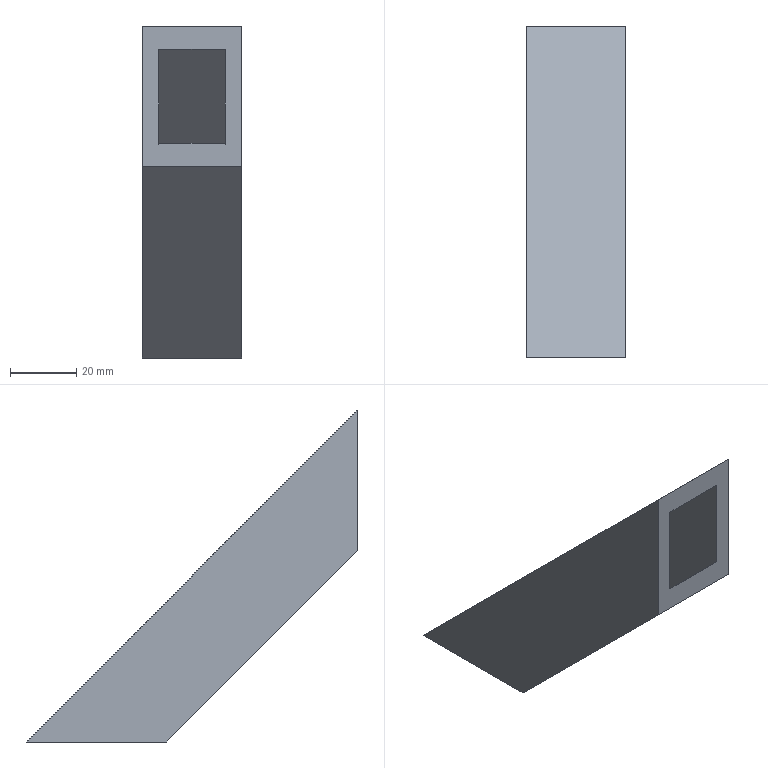Part | NX | features solid 2 | 1 solid | 10 faces | box 30 x 100 x 100 mm | volume 55711 mm3 | plane 10
STEP:
#1=CARTESIAN_POINT('',(-175.,245.,-50.));
#2=VERTEX_POINT('',#1);
#3=CARTESIAN_POINT('',(-205.,245.,-50.));
#4=VERTEX_POINT('',#3);
#5=CARTESIAN_POINT('',(-605.,245.,-50.));
#6=DIRECTION('',(-1.,0.,0.));
#7=VECTOR('',#6,1000.);
#8=LINE('',#5,#7);
#9=EDGE_CURVE('',#2,#4,#8,.T.);
#10=ORIENTED_EDGE('',*,*,#9,.T.);
#11=CARTESIAN_POINT('',(-205.,245.,-92.426));
#12=VERTEX_POINT('',#11);
#13=CARTESIAN_POINT('',(-205.,245.,-92.426));
#14=DIRECTION('',(0.,0.,-1.));
#15=VECTOR('',#14,1000.);
#16=LINE('',#13,#15);
#17=EDGE_CURVE('',#12,#4,#16,.F.);
#18=ORIENTED_EDGE('',*,*,#17,.F.);
#19=CARTESIAN_POINT('',(-175.,245.,-92.426));
#20=VERTEX_POINT('',#19);
#21=CARTESIAN_POINT('',(-175.,245.,-92.426));
#22=DIRECTION('',(1.,0.,0.));
#23=VECTOR('',#22,1000.);
#24=LINE('',#21,#23);
#25=EDGE_CURVE('',#20,#12,#24,.F.);
#26=ORIENTED_EDGE('',*,*,#25,.F.);
#27=CARTESIAN_POINT('',(-175.,245.,-177.426));
#28=DIRECTION('',(0.,0.,1.));
#29=VECTOR('',#28,1000.);
#30=LINE('',#27,#29);
#31=EDGE_CURVE('',#20,#2,#30,.T.);
#32=ORIENTED_EDGE('',*,*,#31,.T.);
#33=EDGE_LOOP('',(#10,#18,#26,#32));
#34=FACE_BOUND('',#33,.T.);
#35=CARTESIAN_POINT('',(-180.,245.,-57.071));
#36=VERTEX_POINT('',#35);
#37=CARTESIAN_POINT('',(-200.,245.,-57.071));
#38=VERTEX_POINT('',#37);
#39=CARTESIAN_POINT('',(-605.,245.,-57.071));
#40=DIRECTION('',(-1.,0.,0.));
#41=VECTOR('',#40,1000.);
#42=LINE('',#39,#41);
#43=EDGE_CURVE('',#36,#38,#42,.T.);
#44=ORIENTED_EDGE('',*,*,#43,.F.);
#45=CARTESIAN_POINT('',(-180.,245.,-85.355));
#46=VERTEX_POINT('',#45);
#47=CARTESIAN_POINT('',(-180.,245.,-177.426));
#48=DIRECTION('',(0.,0.,1.));
#49=VECTOR('',#48,1000.);
#50=LINE('',#47,#49);
#51=EDGE_CURVE('',#46,#36,#50,.T.);
#52=ORIENTED_EDGE('',*,*,#51,.F.);
#53=CARTESIAN_POINT('',(-200.,245.,-85.355));
#54=VERTEX_POINT('',#53);
#55=CARTESIAN_POINT('',(-175.,245.,-85.355));
#56=DIRECTION('',(1.,0.,0.));
#57=VECTOR('',#56,1000.);
#58=LINE('',#55,#57);
#59=EDGE_CURVE('',#46,#54,#58,.F.);
#60=ORIENTED_EDGE('',*,*,#59,.T.);
#61=CARTESIAN_POINT('',(-200.,245.,-92.426));
#62=DIRECTION('',(0.,0.,-1.));
#63=VECTOR('',#62,1000.);
#64=LINE('',#61,#63);
#65=EDGE_CURVE('',#54,#38,#64,.F.);
#66=ORIENTED_EDGE('',*,*,#65,.T.);
#67=EDGE_LOOP('',(#44,#52,#60,#66));
#68=FACE_BOUND('',#67,.T.);
#69=CARTESIAN_POINT('',(-605.,245.,-177.426));
#70=DIRECTION('',(0.,1.,0.));
#71=DIRECTION('',(0.,0.,-1.));
#72=AXIS2_PLACEMENT_3D('',#69,#70,#71);
#73=PLANE('',#72);
#74=ADVANCED_FACE('',(#34,#68),#73,.F.);
#75=CARTESIAN_POINT('',(-205.,302.574,-150.));
#76=VERTEX_POINT('',#75);
#77=CARTESIAN_POINT('',(-205.,245.,-92.426));
#78=DIRECTION('',(0.,0.7071,-0.7071));
#79=VECTOR('',#78,1000.);
#80=LINE('',#77,#79);
#81=EDGE_CURVE('',#76,#12,#80,.F.);
#82=ORIENTED_EDGE('',*,*,#81,.F.);
#83=CARTESIAN_POINT('',(-175.,302.574,-150.));
#84=VERTEX_POINT('',#83);
#85=CARTESIAN_POINT('',(-175.,302.574,-150.));
#86=DIRECTION('',(1.,0.,0.));
#87=VECTOR('',#86,1000.);
#88=LINE('',#85,#87);
#89=EDGE_CURVE('',#76,#84,#88,.T.);
#90=ORIENTED_EDGE('',*,*,#89,.T.);
#91=CARTESIAN_POINT('',(-175.,245.,-92.426));
#92=DIRECTION('',(0.,0.7071,-0.7071));
#93=VECTOR('',#92,1000.);
#94=LINE('',#91,#93);
#95=EDGE_CURVE('',#84,#20,#94,.F.);
#96=ORIENTED_EDGE('',*,*,#95,.T.);
#97=ORIENTED_EDGE('',*,*,#25,.T.);
#98=EDGE_LOOP('',(#82,#90,#96,#97));
#99=FACE_BOUND('',#98,.T.);
#100=CARTESIAN_POINT('',(-175.,245.,-92.426));
#101=DIRECTION('',(0.,-0.7071,-0.7071));
#102=DIRECTION('',(-1.,0.,0.));
#103=AXIS2_PLACEMENT_3D('',#100,#101,#102);
#104=PLANE('',#103);
#105=ADVANCED_FACE('',(#99),#104,.T.);
#106=CARTESIAN_POINT('',(-205.,345.,-150.));
#107=VERTEX_POINT('',#106);
#108=CARTESIAN_POINT('',(-205.,266.213,-71.213));
#109=DIRECTION('',(0.,0.7071,-0.7071));
#110=VECTOR('',#109,1000.);
#111=LINE('',#108,#110);
#112=EDGE_CURVE('',#107,#4,#111,.F.);
#113=ORIENTED_EDGE('',*,*,#112,.F.);
#114=CARTESIAN_POINT('',(-205.,245.,-150.));
#115=DIRECTION('',(0.,-1.,0.));
#116=VECTOR('',#115,1000.);
#117=LINE('',#114,#116);
#118=EDGE_CURVE('',#107,#76,#117,.T.);
#119=ORIENTED_EDGE('',*,*,#118,.T.);
#120=ORIENTED_EDGE('',*,*,#81,.T.);
#121=ORIENTED_EDGE('',*,*,#17,.T.);
#122=EDGE_LOOP('',(#113,#119,#120,#121));
#123=FACE_BOUND('',#122,.T.);
#124=CARTESIAN_POINT('',(-205.,245.,-92.426));
#125=DIRECTION('',(-1.,0.,0.));
#126=DIRECTION('',(0.,0.7071,0.7071));
#127=AXIS2_PLACEMENT_3D('',#124,#125,#126);
#128=PLANE('',#127);
#129=ADVANCED_FACE('',(#123),#128,.T.);
#130=CARTESIAN_POINT('',(-175.,345.,-150.));
#131=VERTEX_POINT('',#130);
#132=CARTESIAN_POINT('',(-175.,266.213,-71.213));
#133=DIRECTION('',(0.,0.7071,-0.7071));
#134=VECTOR('',#133,1000.);
#135=LINE('',#132,#134);
#136=EDGE_CURVE('',#131,#2,#135,.F.);
#137=ORIENTED_EDGE('',*,*,#136,.F.);
#138=CARTESIAN_POINT('',(-175.,345.,-150.));
#139=DIRECTION('',(1.,0.,0.));
#140=VECTOR('',#139,1000.);
#141=LINE('',#138,#140);
#142=EDGE_CURVE('',#131,#107,#141,.F.);
#143=ORIENTED_EDGE('',*,*,#142,.T.);
#144=ORIENTED_EDGE('',*,*,#112,.T.);
#145=ORIENTED_EDGE('',*,*,#9,.F.);
#146=EDGE_LOOP('',(#137,#143,#144,#145));
#147=FACE_BOUND('',#146,.T.);
#148=CARTESIAN_POINT('',(-175.,266.213,-71.213));
#149=DIRECTION('',(0.,-0.7071,-0.7071));
#150=DIRECTION('',(-1.,0.,0.));
#151=AXIS2_PLACEMENT_3D('',#148,#149,#150);
#152=PLANE('',#151);
#153=ADVANCED_FACE('',(#147),#152,.F.);
#154=ORIENTED_EDGE('',*,*,#95,.F.);
#155=CARTESIAN_POINT('',(-175.,245.,-150.));
#156=DIRECTION('',(0.,-1.,0.));
#157=VECTOR('',#156,1000.);
#158=LINE('',#155,#157);
#159=EDGE_CURVE('',#84,#131,#158,.F.);
#160=ORIENTED_EDGE('',*,*,#159,.T.);
#161=ORIENTED_EDGE('',*,*,#136,.T.);
#162=ORIENTED_EDGE('',*,*,#31,.F.);
#163=EDGE_LOOP('',(#154,#160,#161,#162));
#164=FACE_BOUND('',#163,.T.);
#165=CARTESIAN_POINT('',(-175.,245.,-92.426));
#166=DIRECTION('',(-1.,0.,0.));
#167=DIRECTION('',(0.,0.7071,0.7071));
#168=AXIS2_PLACEMENT_3D('',#165,#166,#167);
#169=PLANE('',#168);
#170=ADVANCED_FACE('',(#164),#169,.F.);
#171=CARTESIAN_POINT('',(-200.,309.645,-150.));
#172=VERTEX_POINT('',#171);
#173=CARTESIAN_POINT('',(-180.,309.645,-150.));
#174=VERTEX_POINT('',#173);
#175=CARTESIAN_POINT('',(-175.,309.645,-150.));
#176=DIRECTION('',(1.,0.,0.));
#177=VECTOR('',#176,1000.);
#178=LINE('',#175,#177);
#179=EDGE_CURVE('',#172,#174,#178,.T.);
#180=ORIENTED_EDGE('',*,*,#179,.F.);
#181=CARTESIAN_POINT('',(-200.,248.536,-88.891));
#182=DIRECTION('',(0.,-0.7071,0.7071));
#183=VECTOR('',#182,1000.);
#184=LINE('',#181,#183);
#185=EDGE_CURVE('',#172,#54,#184,.T.);
#186=ORIENTED_EDGE('',*,*,#185,.T.);
#187=ORIENTED_EDGE('',*,*,#59,.F.);
#188=CARTESIAN_POINT('',(-180.,248.536,-88.891));
#189=DIRECTION('',(0.,0.7071,-0.7071));
#190=VECTOR('',#189,1000.);
#191=LINE('',#188,#190);
#192=EDGE_CURVE('',#174,#46,#191,.F.);
#193=ORIENTED_EDGE('',*,*,#192,.F.);
#194=EDGE_LOOP('',(#180,#186,#187,#193));
#195=FACE_BOUND('',#194,.T.);
#196=CARTESIAN_POINT('',(-175.,248.536,-88.891));
#197=DIRECTION('',(0.,-0.7071,-0.7071));
#198=DIRECTION('',(-1.,0.,0.));
#199=AXIS2_PLACEMENT_3D('',#196,#197,#198);
#200=PLANE('',#199);
#201=ADVANCED_FACE('',(#195),#200,.F.);
#202=CARTESIAN_POINT('',(-200.,337.929,-150.));
#203=VERTEX_POINT('',#202);
#204=CARTESIAN_POINT('',(-200.,245.,-150.));
#205=DIRECTION('',(0.,-1.,0.));
#206=VECTOR('',#205,1000.);
#207=LINE('',#204,#206);
#208=EDGE_CURVE('',#203,#172,#207,.T.);
#209=ORIENTED_EDGE('',*,*,#208,.F.);
#210=CARTESIAN_POINT('',(-200.,262.678,-74.749));
#211=DIRECTION('',(0.,0.7071,-0.7071));
#212=VECTOR('',#211,1000.);
#213=LINE('',#210,#212);
#214=EDGE_CURVE('',#203,#38,#213,.F.);
#215=ORIENTED_EDGE('',*,*,#214,.T.);
#216=ORIENTED_EDGE('',*,*,#65,.F.);
#217=ORIENTED_EDGE('',*,*,#185,.F.);
#218=EDGE_LOOP('',(#209,#215,#216,#217));
#219=FACE_BOUND('',#218,.T.);
#220=CARTESIAN_POINT('',(-200.,245.,-92.426));
#221=DIRECTION('',(-1.,0.,0.));
#222=DIRECTION('',(0.,0.7071,0.7071));
#223=AXIS2_PLACEMENT_3D('',#220,#221,#222);
#224=PLANE('',#223);
#225=ADVANCED_FACE('',(#219),#224,.F.);
#226=CARTESIAN_POINT('',(-180.,337.929,-150.));
#227=VERTEX_POINT('',#226);
#228=CARTESIAN_POINT('',(-175.,337.929,-150.));
#229=DIRECTION('',(1.,0.,0.));
#230=VECTOR('',#229,1000.);
#231=LINE('',#228,#230);
#232=EDGE_CURVE('',#227,#203,#231,.F.);
#233=ORIENTED_EDGE('',*,*,#232,.F.);
#234=CARTESIAN_POINT('',(-180.,262.678,-74.749));
#235=DIRECTION('',(0.,-0.7071,0.7071));
#236=VECTOR('',#235,1000.);
#237=LINE('',#234,#236);
#238=EDGE_CURVE('',#227,#36,#237,.T.);
#239=ORIENTED_EDGE('',*,*,#238,.T.);
#240=ORIENTED_EDGE('',*,*,#43,.T.);
#241=ORIENTED_EDGE('',*,*,#214,.F.);
#242=EDGE_LOOP('',(#233,#239,#240,#241));
#243=FACE_BOUND('',#242,.T.);
#244=CARTESIAN_POINT('',(-175.,262.678,-74.749));
#245=DIRECTION('',(0.,-0.7071,-0.7071));
#246=DIRECTION('',(-1.,0.,0.));
#247=AXIS2_PLACEMENT_3D('',#244,#245,#246);
#248=PLANE('',#247);
#249=ADVANCED_FACE('',(#243),#248,.T.);
#250=CARTESIAN_POINT('',(-180.,245.,-150.));
#251=DIRECTION('',(0.,-1.,0.));
#252=VECTOR('',#251,1000.);
#253=LINE('',#250,#252);
#254=EDGE_CURVE('',#174,#227,#253,.F.);
#255=ORIENTED_EDGE('',*,*,#254,.F.);
#256=ORIENTED_EDGE('',*,*,#192,.T.);
#257=ORIENTED_EDGE('',*,*,#51,.T.);
#258=ORIENTED_EDGE('',*,*,#238,.F.);
#259=EDGE_LOOP('',(#255,#256,#257,#258));
#260=FACE_BOUND('',#259,.T.);
#261=CARTESIAN_POINT('',(-180.,245.,-92.426));
#262=DIRECTION('',(-1.,0.,0.));
#263=DIRECTION('',(0.,0.7071,0.7071));
#264=AXIS2_PLACEMENT_3D('',#261,#262,#263);
#265=PLANE('',#264);
#266=ADVANCED_FACE('',(#260),#265,.T.);
#267=ORIENTED_EDGE('',*,*,#179,.T.);
#268=ORIENTED_EDGE('',*,*,#254,.T.);
#269=ORIENTED_EDGE('',*,*,#232,.T.);
#270=ORIENTED_EDGE('',*,*,#208,.T.);
#271=EDGE_LOOP('',(#267,#268,#269,#270));
#272=FACE_BOUND('',#271,.T.);
#273=ORIENTED_EDGE('',*,*,#118,.F.);
#274=ORIENTED_EDGE('',*,*,#142,.F.);
#275=ORIENTED_EDGE('',*,*,#159,.F.);
#276=ORIENTED_EDGE('',*,*,#89,.F.);
#277=EDGE_LOOP('',(#273,#274,#275,#276));
#278=FACE_BOUND('',#277,.T.);
#279=CARTESIAN_POINT('',(-175.,295.,-150.));
#280=DIRECTION('',(0.,0.,-1.));
#281=DIRECTION('',(-1.,0.,0.));
#282=AXIS2_PLACEMENT_3D('',#279,#280,#281);
#283=PLANE('',#282);
#284=ADVANCED_FACE('',(#272,#278),#283,.T.);
#285=CLOSED_SHELL('',(#74,#105,#129,#153,#170,#201,#225,#249,#266,#284));
#286=MANIFOLD_SOLID_BREP('',#285);
#287=(LENGTH_UNIT()NAMED_UNIT(*)SI_UNIT(.MILLI.,.METRE.));
#288=UNCERTAINTY_MEASURE_WITH_UNIT(LENGTH_MEASURE(0.00001),#287,'','');
#289=(NAMED_UNIT(*)PLANE_ANGLE_UNIT()SI_UNIT($,.RADIAN.));
#290=(NAMED_UNIT(*)SI_UNIT($,.STERADIAN.)SOLID_ANGLE_UNIT());
#291=(GEOMETRIC_REPRESENTATION_CONTEXT(3)GLOBAL_UNCERTAINTY_ASSIGNED_CONTEXT((#288))GLOBAL_UNIT_ASSIGNED_CONTEXT((#287,#289,#290))REPRESENTATION_CONTEXT('',''));
#292=ADVANCED_BREP_SHAPE_REPRESENTATION('',(#286),#291);